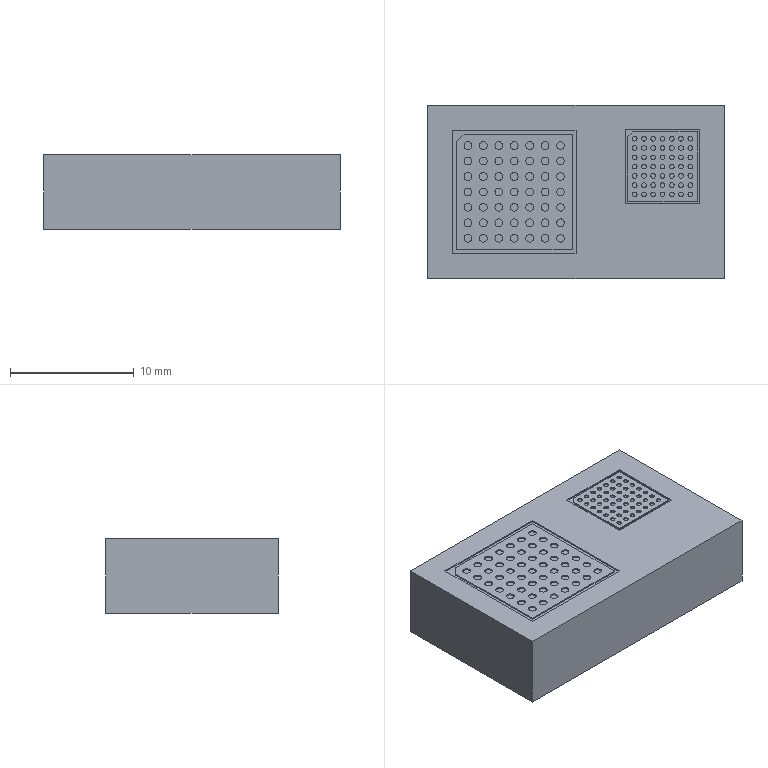Part | STEP file | ASND-0110-TPIM-标定01 | 1 solid | 322 faces | box 24 x 14 x 6 mm | volume 2012 mm3 | cylinder 196 | plane 126 | commonest cylinder face diameters 0.375 x98 0.625 x98